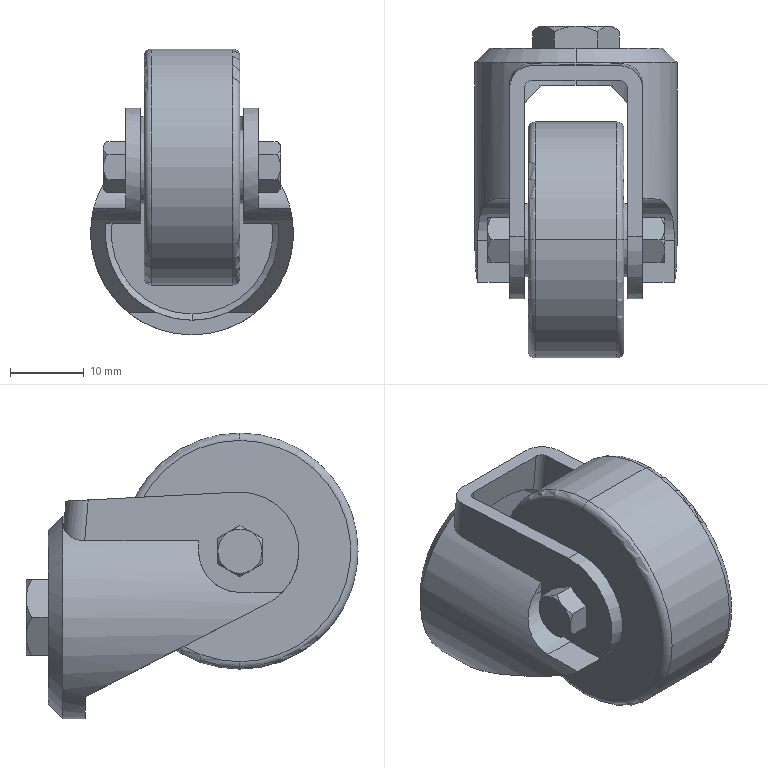Part | SolidWorks | features ICE 3, BaseBody 2 | 1 solid | 94 faces | box 27.5 x 45 x 38.75 mm | volume 15003 mm3 | plane 44 | cone 24 | cylinder 22 | torus 4 | commonest cylinder face diameters 10 x4 2 x2 6 x2 8 x2 11.2 x2 15.2 x2